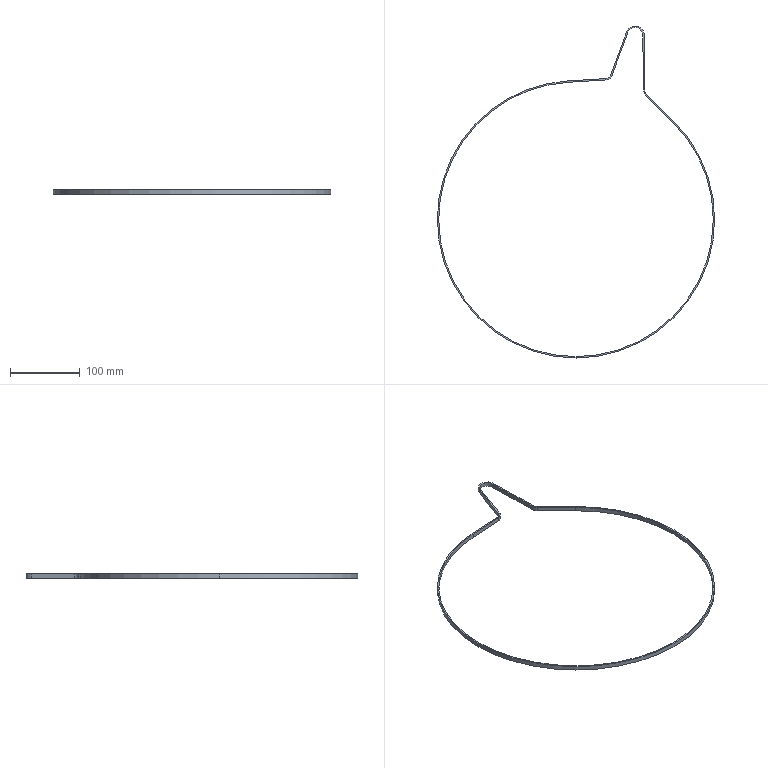Part | NX | features BREP 1 | 1 solid | 22 faces | box 398.69 x 477.38 x 6 mm | volume 16623 mm3 | cylinder 12 | plane 10 | commonest cylinder face diameters 394.69 x3 398.69 x3 17 x2 21 x2 22.07 x1 26.07 x1
STEP:
#1=CARTESIAN_POINT('',(42.641,200.38,-3.));
#2=VERTEX_POINT('',#1);
#3=CARTESIAN_POINT('',(-12.257,196.964,-3.));
#4=VERTEX_POINT('',#3);
#5=CARTESIAN_POINT('',(-12.257,196.964,-3.));
#6=DIRECTION('',(-0.9981,-0.06211,0.));
#7=VECTOR('',#6,1000.);
#8=LINE('',#5,#7);
#9=EDGE_CURVE('',#2,#4,#8,.T.);
#10=ORIENTED_EDGE('',*,*,#9,.F.);
#11=CARTESIAN_POINT('',(42.641,200.38,3.));
#12=VERTEX_POINT('',#11);
#13=CARTESIAN_POINT('',(42.641,200.38,3.));
#14=DIRECTION('',(0.,0.,-1.));
#15=VECTOR('',#14,1000.);
#16=LINE('',#13,#15);
#17=EDGE_CURVE('',#12,#2,#16,.T.);
#18=ORIENTED_EDGE('',*,*,#17,.F.);
#19=CARTESIAN_POINT('',(-12.257,196.964,3.));
#20=VERTEX_POINT('',#19);
#21=CARTESIAN_POINT('',(-12.257,196.964,3.));
#22=DIRECTION('',(-0.9981,-0.06211,0.));
#23=VECTOR('',#22,1000.);
#24=LINE('',#21,#23);
#25=EDGE_CURVE('',#12,#20,#24,.T.);
#26=ORIENTED_EDGE('',*,*,#25,.T.);
#27=CARTESIAN_POINT('',(-12.257,196.964,3.));
#28=DIRECTION('',(0.,0.,-1.));
#29=VECTOR('',#28,1000.);
#30=LINE('',#27,#29);
#31=EDGE_CURVE('',#20,#4,#30,.T.);
#32=ORIENTED_EDGE('',*,*,#31,.T.);
#33=EDGE_LOOP('',(#10,#18,#26,#32));
#34=FACE_BOUND('',#33,.T.);
#35=CARTESIAN_POINT('',(-12.257,196.964,3.));
#36=DIRECTION('',(0.06211,-0.9981,0.));
#37=DIRECTION('',(0.9981,0.06211,0.));
#38=AXIS2_PLACEMENT_3D('',#35,#36,#37);
#39=PLANE('',#38);
#40=ADVANCED_FACE('',(#34),#39,.T.);
#41=CARTESIAN_POINT('',(51.836,207.214,-3.));
#42=VERTEX_POINT('',#41);
#43=CARTESIAN_POINT('',(41.989,210.86,-3.));
#44=DIRECTION('',(0.,0.,-1.));
#45=DIRECTION('',(-1.,0.,0.));
#46=AXIS2_PLACEMENT_3D('',#43,#44,#45);
#47=CIRCLE('',#46,10.5);
#48=EDGE_CURVE('',#42,#2,#47,.T.);
#49=ORIENTED_EDGE('',*,*,#48,.F.);
#50=CARTESIAN_POINT('',(51.836,207.214,3.));
#51=VERTEX_POINT('',#50);
#52=CARTESIAN_POINT('',(51.836,207.214,3.));
#53=DIRECTION('',(0.,0.,-1.));
#54=VECTOR('',#53,1000.);
#55=LINE('',#52,#54);
#56=EDGE_CURVE('',#51,#42,#55,.T.);
#57=ORIENTED_EDGE('',*,*,#56,.F.);
#58=CARTESIAN_POINT('',(41.989,210.86,3.));
#59=DIRECTION('',(0.,0.,-1.));
#60=DIRECTION('',(-1.,0.,0.));
#61=AXIS2_PLACEMENT_3D('',#58,#59,#60);
#62=CIRCLE('',#61,10.5);
#63=EDGE_CURVE('',#51,#12,#62,.T.);
#64=ORIENTED_EDGE('',*,*,#63,.T.);
#65=ORIENTED_EDGE('',*,*,#17,.T.);
#66=EDGE_LOOP('',(#49,#57,#64,#65));
#67=FACE_BOUND('',#66,.T.);
#68=CARTESIAN_POINT('',(41.989,210.86,3.));
#69=DIRECTION('',(0.,0.,-1.));
#70=DIRECTION('',(-1.,0.,0.));
#71=AXIS2_PLACEMENT_3D('',#68,#69,#70);
#72=CYLINDRICAL_SURFACE('',#71,10.5);
#73=ADVANCED_FACE('',(#67),#72,.T.);
#74=CARTESIAN_POINT('',(74.652,268.832,-3.));
#75=VERTEX_POINT('',#74);
#76=CARTESIAN_POINT('',(-21.89,8.105,-3.));
#77=DIRECTION('',(-0.3472,-0.9378,0.));
#78=VECTOR('',#77,1000.);
#79=LINE('',#76,#78);
#80=EDGE_CURVE('',#75,#42,#79,.T.);
#81=ORIENTED_EDGE('',*,*,#80,.F.);
#82=CARTESIAN_POINT('',(74.652,268.832,3.));
#83=VERTEX_POINT('',#82);
#84=CARTESIAN_POINT('',(74.652,268.832,3.));
#85=DIRECTION('',(0.,0.,-1.));
#86=VECTOR('',#85,1000.);
#87=LINE('',#84,#86);
#88=EDGE_CURVE('',#83,#75,#87,.T.);
#89=ORIENTED_EDGE('',*,*,#88,.F.);
#90=CARTESIAN_POINT('',(-21.89,8.105,3.));
#91=DIRECTION('',(-0.3472,-0.9378,0.));
#92=VECTOR('',#91,1000.);
#93=LINE('',#90,#92);
#94=EDGE_CURVE('',#83,#51,#93,.T.);
#95=ORIENTED_EDGE('',*,*,#94,.T.);
#96=ORIENTED_EDGE('',*,*,#56,.T.);
#97=EDGE_LOOP('',(#81,#89,#95,#96));
#98=FACE_BOUND('',#97,.T.);
#99=CARTESIAN_POINT('',(-21.89,8.105,3.));
#100=DIRECTION('',(0.9378,-0.3472,0.));
#101=DIRECTION('',(0.3472,0.9378,0.));
#102=AXIS2_PLACEMENT_3D('',#99,#100,#101);
#103=PLANE('',#102);
#104=ADVANCED_FACE('',(#98),#103,.T.);
#105=CARTESIAN_POINT('',(96.034,265.135,-3.));
#106=VERTEX_POINT('',#105);
#107=CARTESIAN_POINT('',(85.,265.,-3.));
#108=DIRECTION('',(0.,0.,1.));
#109=DIRECTION('',(-1.,0.,0.));
#110=AXIS2_PLACEMENT_3D('',#107,#108,#109);
#111=CIRCLE('',#110,11.035);
#112=EDGE_CURVE('',#106,#75,#111,.T.);
#113=ORIENTED_EDGE('',*,*,#112,.F.);
#114=CARTESIAN_POINT('',(96.034,265.135,3.));
#115=VERTEX_POINT('',#114);
#116=CARTESIAN_POINT('',(96.034,265.135,3.));
#117=DIRECTION('',(0.,0.,-1.));
#118=VECTOR('',#117,1000.);
#119=LINE('',#116,#118);
#120=EDGE_CURVE('',#115,#106,#119,.T.);
#121=ORIENTED_EDGE('',*,*,#120,.F.);
#122=CARTESIAN_POINT('',(85.,265.,3.));
#123=DIRECTION('',(0.,0.,1.));
#124=DIRECTION('',(-1.,0.,0.));
#125=AXIS2_PLACEMENT_3D('',#122,#123,#124);
#126=CIRCLE('',#125,11.035);
#127=EDGE_CURVE('',#115,#83,#126,.T.);
#128=ORIENTED_EDGE('',*,*,#127,.T.);
#129=ORIENTED_EDGE('',*,*,#88,.T.);
#130=EDGE_LOOP('',(#113,#121,#128,#129));
#131=FACE_BOUND('',#130,.T.);
#132=CARTESIAN_POINT('',(85.,265.,3.));
#133=DIRECTION('',(0.,0.,-1.));
#134=DIRECTION('',(-1.,0.,0.));
#135=AXIS2_PLACEMENT_3D('',#132,#133,#134);
#136=CYLINDRICAL_SURFACE('',#135,11.035);
#137=ADVANCED_FACE('',(#131),#136,.F.);
#138=CARTESIAN_POINT('',(97.001,186.067,-3.));
#139=VERTEX_POINT('',#138);
#140=CARTESIAN_POINT('',(99.261,1.213,-3.));
#141=DIRECTION('',(-0.01222,0.9999,0.));
#142=VECTOR('',#141,1000.);
#143=LINE('',#140,#142);
#144=EDGE_CURVE('',#139,#106,#143,.T.);
#145=ORIENTED_EDGE('',*,*,#144,.F.);
#146=CARTESIAN_POINT('',(97.001,186.067,3.));
#147=VERTEX_POINT('',#146);
#148=CARTESIAN_POINT('',(97.001,186.067,3.));
#149=DIRECTION('',(0.,0.,-1.));
#150=VECTOR('',#149,1000.);
#151=LINE('',#148,#150);
#152=EDGE_CURVE('',#147,#139,#151,.T.);
#153=ORIENTED_EDGE('',*,*,#152,.F.);
#154=CARTESIAN_POINT('',(99.261,1.213,3.));
#155=DIRECTION('',(-0.01222,0.9999,0.));
#156=VECTOR('',#155,1000.);
#157=LINE('',#154,#156);
#158=EDGE_CURVE('',#147,#115,#157,.T.);
#159=ORIENTED_EDGE('',*,*,#158,.T.);
#160=ORIENTED_EDGE('',*,*,#120,.T.);
#161=EDGE_LOOP('',(#145,#153,#159,#160));
#162=FACE_BOUND('',#161,.T.);
#163=CARTESIAN_POINT('',(99.261,1.213,3.));
#164=DIRECTION('',(-0.9999,-0.01222,0.));
#165=DIRECTION('',(0.01222,-0.9999,0.));
#166=AXIS2_PLACEMENT_3D('',#163,#164,#165);
#167=PLANE('',#166);
#168=ADVANCED_FACE('',(#162),#167,.T.);
#169=CARTESIAN_POINT('',(100.098,178.748,-3.));
#170=VERTEX_POINT('',#169);
#171=CARTESIAN_POINT('',(107.5,186.195,-3.));
#172=DIRECTION('',(0.,0.,-1.));
#173=DIRECTION('',(-1.,0.,0.));
#174=AXIS2_PLACEMENT_3D('',#171,#172,#173);
#175=CIRCLE('',#174,10.5);
#176=EDGE_CURVE('',#170,#139,#175,.T.);
#177=ORIENTED_EDGE('',*,*,#176,.F.);
#178=CARTESIAN_POINT('',(100.098,178.748,3.));
#179=VERTEX_POINT('',#178);
#180=CARTESIAN_POINT('',(100.098,178.748,3.));
#181=DIRECTION('',(0.,0.,-1.));
#182=VECTOR('',#181,1000.);
#183=LINE('',#180,#182);
#184=EDGE_CURVE('',#179,#170,#183,.T.);
#185=ORIENTED_EDGE('',*,*,#184,.F.);
#186=CARTESIAN_POINT('',(107.5,186.195,3.));
#187=DIRECTION('',(0.,0.,-1.));
#188=DIRECTION('',(-1.,0.,0.));
#189=AXIS2_PLACEMENT_3D('',#186,#187,#188);
#190=CIRCLE('',#189,10.5);
#191=EDGE_CURVE('',#179,#147,#190,.T.);
#192=ORIENTED_EDGE('',*,*,#191,.T.);
#193=ORIENTED_EDGE('',*,*,#152,.T.);
#194=EDGE_LOOP('',(#177,#185,#192,#193));
#195=FACE_BOUND('',#194,.T.);
#196=CARTESIAN_POINT('',(107.5,186.195,3.));
#197=DIRECTION('',(0.,0.,-1.));
#198=DIRECTION('',(-1.,0.,0.));
#199=AXIS2_PLACEMENT_3D('',#196,#197,#198);
#200=CYLINDRICAL_SURFACE('',#199,10.5);
#201=ADVANCED_FACE('',(#195),#200,.T.);
#202=CARTESIAN_POINT('',(139.112,139.974,-3.));
#203=VERTEX_POINT('',#202);
#204=CARTESIAN_POINT('',(139.112,139.974,-3.));
#205=DIRECTION('',(-0.7093,0.7049,0.));
#206=VECTOR('',#205,1000.);
#207=LINE('',#204,#206);
#208=EDGE_CURVE('',#203,#170,#207,.T.);
#209=ORIENTED_EDGE('',*,*,#208,.F.);
#210=CARTESIAN_POINT('',(139.112,139.974,3.));
#211=VERTEX_POINT('',#210);
#212=CARTESIAN_POINT('',(139.112,139.974,3.));
#213=DIRECTION('',(0.,0.,-1.));
#214=VECTOR('',#213,1000.);
#215=LINE('',#212,#214);
#216=EDGE_CURVE('',#211,#203,#215,.T.);
#217=ORIENTED_EDGE('',*,*,#216,.F.);
#218=CARTESIAN_POINT('',(139.112,139.974,3.));
#219=DIRECTION('',(-0.7093,0.7049,0.));
#220=VECTOR('',#219,1000.);
#221=LINE('',#218,#220);
#222=EDGE_CURVE('',#211,#179,#221,.T.);
#223=ORIENTED_EDGE('',*,*,#222,.T.);
#224=ORIENTED_EDGE('',*,*,#184,.T.);
#225=EDGE_LOOP('',(#209,#217,#223,#224));
#226=FACE_BOUND('',#225,.T.);
#227=CARTESIAN_POINT('',(139.112,139.974,3.));
#228=DIRECTION('',(-0.7049,-0.7093,0.));
#229=DIRECTION('',(0.7093,-0.7049,0.));
#230=AXIS2_PLACEMENT_3D('',#227,#228,#229);
#231=PLANE('',#230);
#232=ADVANCED_FACE('',(#226),#231,.T.);
#233=CARTESIAN_POINT('',(197.345,0.,3.));
#234=VERTEX_POINT('',#233);
#235=CARTESIAN_POINT('',(197.345,0.,-3.));
#236=VERTEX_POINT('',#235);
#237=CARTESIAN_POINT('',(197.345,0.,3.));
#238=DIRECTION('',(0.,0.,-1.));
#239=VECTOR('',#238,1000.);
#240=LINE('',#237,#239);
#241=EDGE_CURVE('',#234,#236,#240,.T.);
#242=ORIENTED_EDGE('',*,*,#241,.F.);
#243=CARTESIAN_POINT('',(0.,0.,3.));
#244=DIRECTION('',(0.,0.,1.));
#245=DIRECTION('',(-1.,0.,0.));
#246=AXIS2_PLACEMENT_3D('',#243,#244,#245);
#247=CIRCLE('',#246,197.345);
#248=EDGE_CURVE('',#234,#211,#247,.T.);
#249=ORIENTED_EDGE('',*,*,#248,.T.);
#250=ORIENTED_EDGE('',*,*,#216,.T.);
#251=CARTESIAN_POINT('',(0.,0.,-3.));
#252=DIRECTION('',(0.,0.,1.));
#253=DIRECTION('',(-1.,0.,0.));
#254=AXIS2_PLACEMENT_3D('',#251,#252,#253);
#255=CIRCLE('',#254,197.345);
#256=EDGE_CURVE('',#236,#203,#255,.T.);
#257=ORIENTED_EDGE('',*,*,#256,.F.);
#258=EDGE_LOOP('',(#242,#249,#250,#257));
#259=FACE_BOUND('',#258,.T.);
#260=CARTESIAN_POINT('',(0.,0.,3.));
#261=DIRECTION('',(0.,0.,-1.));
#262=DIRECTION('',(-1.,0.,0.));
#263=AXIS2_PLACEMENT_3D('',#260,#261,#262);
#264=CYLINDRICAL_SURFACE('',#263,197.345);
#265=ADVANCED_FACE('',(#259),#264,.F.);
#266=CARTESIAN_POINT('',(42.517,202.376,-3.));
#267=VERTEX_POINT('',#266);
#268=CARTESIAN_POINT('',(-12.381,198.96,-3.));
#269=VERTEX_POINT('',#268);
#270=CARTESIAN_POINT('',(-12.381,198.96,-3.));
#271=DIRECTION('',(-0.9981,-0.06211,0.));
#272=VECTOR('',#271,1000.);
#273=LINE('',#270,#272);
#274=EDGE_CURVE('',#267,#269,#273,.T.);
#275=ORIENTED_EDGE('',*,*,#274,.T.);
#276=CARTESIAN_POINT('',(-12.381,198.96,3.));
#277=VERTEX_POINT('',#276);
#278=CARTESIAN_POINT('',(-12.381,198.96,3.));
#279=DIRECTION('',(0.,0.,-1.));
#280=VECTOR('',#279,1000.);
#281=LINE('',#278,#280);
#282=EDGE_CURVE('',#277,#269,#281,.T.);
#283=ORIENTED_EDGE('',*,*,#282,.F.);
#284=CARTESIAN_POINT('',(42.517,202.376,3.));
#285=VERTEX_POINT('',#284);
#286=CARTESIAN_POINT('',(-12.381,198.96,3.));
#287=DIRECTION('',(-0.9981,-0.06211,0.));
#288=VECTOR('',#287,1000.);
#289=LINE('',#286,#288);
#290=EDGE_CURVE('',#285,#277,#289,.T.);
#291=ORIENTED_EDGE('',*,*,#290,.F.);
#292=CARTESIAN_POINT('',(42.517,202.376,3.));
#293=DIRECTION('',(0.,0.,-1.));
#294=VECTOR('',#293,1000.);
#295=LINE('',#292,#294);
#296=EDGE_CURVE('',#285,#267,#295,.T.);
#297=ORIENTED_EDGE('',*,*,#296,.T.);
#298=EDGE_LOOP('',(#275,#283,#291,#297));
#299=FACE_BOUND('',#298,.T.);
#300=CARTESIAN_POINT('',(-12.381,198.96,3.));
#301=DIRECTION('',(0.06211,-0.9981,0.));
#302=DIRECTION('',(0.9981,0.06211,0.));
#303=AXIS2_PLACEMENT_3D('',#300,#301,#302);
#304=PLANE('',#303);
#305=ADVANCED_FACE('',(#299),#304,.F.);
#306=CARTESIAN_POINT('',(49.96,207.908,-3.));
#307=VERTEX_POINT('',#306);
#308=CARTESIAN_POINT('',(41.989,210.86,-3.));
#309=DIRECTION('',(0.,0.,-1.));
#310=DIRECTION('',(-1.,0.,0.));
#311=AXIS2_PLACEMENT_3D('',#308,#309,#310);
#312=CIRCLE('',#311,8.5);
#313=EDGE_CURVE('',#307,#267,#312,.T.);
#314=ORIENTED_EDGE('',*,*,#313,.T.);
#315=ORIENTED_EDGE('',*,*,#296,.F.);
#316=CARTESIAN_POINT('',(49.96,207.908,3.));
#317=VERTEX_POINT('',#316);
#318=CARTESIAN_POINT('',(41.989,210.86,3.));
#319=DIRECTION('',(0.,0.,-1.));
#320=DIRECTION('',(-1.,0.,0.));
#321=AXIS2_PLACEMENT_3D('',#318,#319,#320);
#322=CIRCLE('',#321,8.5);
#323=EDGE_CURVE('',#317,#285,#322,.T.);
#324=ORIENTED_EDGE('',*,*,#323,.F.);
#325=CARTESIAN_POINT('',(49.96,207.908,3.));
#326=DIRECTION('',(0.,0.,-1.));
#327=VECTOR('',#326,1000.);
#328=LINE('',#325,#327);
#329=EDGE_CURVE('',#317,#307,#328,.T.);
#330=ORIENTED_EDGE('',*,*,#329,.T.);
#331=EDGE_LOOP('',(#314,#315,#324,#330));
#332=FACE_BOUND('',#331,.T.);
#333=CARTESIAN_POINT('',(41.989,210.86,3.));
#334=DIRECTION('',(0.,0.,-1.));
#335=DIRECTION('',(-1.,0.,0.));
#336=AXIS2_PLACEMENT_3D('',#333,#334,#335);
#337=CYLINDRICAL_SURFACE('',#336,8.5);
#338=ADVANCED_FACE('',(#332),#337,.F.);
#339=CARTESIAN_POINT('',(72.776,269.526,-3.));
#340=VERTEX_POINT('',#339);
#341=CARTESIAN_POINT('',(-23.765,8.8,-3.));
#342=DIRECTION('',(-0.3472,-0.9378,0.));
#343=VECTOR('',#342,1000.);
#344=LINE('',#341,#343);
#345=EDGE_CURVE('',#340,#307,#344,.T.);
#346=ORIENTED_EDGE('',*,*,#345,.T.);
#347=ORIENTED_EDGE('',*,*,#329,.F.);
#348=CARTESIAN_POINT('',(72.776,269.526,3.));
#349=VERTEX_POINT('',#348);
#350=CARTESIAN_POINT('',(-23.765,8.8,3.));
#351=DIRECTION('',(-0.3472,-0.9378,0.));
#352=VECTOR('',#351,1000.);
#353=LINE('',#350,#352);
#354=EDGE_CURVE('',#349,#317,#353,.T.);
#355=ORIENTED_EDGE('',*,*,#354,.F.);
#356=CARTESIAN_POINT('',(72.776,269.526,3.));
#357=DIRECTION('',(0.,0.,-1.));
#358=VECTOR('',#357,1000.);
#359=LINE('',#356,#358);
#360=EDGE_CURVE('',#349,#340,#359,.T.);
#361=ORIENTED_EDGE('',*,*,#360,.T.);
#362=EDGE_LOOP('',(#346,#347,#355,#361));
#363=FACE_BOUND('',#362,.T.);
#364=CARTESIAN_POINT('',(-23.765,8.8,3.));
#365=DIRECTION('',(0.9378,-0.3472,0.));
#366=DIRECTION('',(0.3472,0.9378,0.));
#367=AXIS2_PLACEMENT_3D('',#364,#365,#366);
#368=PLANE('',#367);
#369=ADVANCED_FACE('',(#363),#368,.F.);
#370=CARTESIAN_POINT('',(98.034,265.159,-3.));
#371=VERTEX_POINT('',#370);
#372=CARTESIAN_POINT('',(85.,265.,-3.));
#373=DIRECTION('',(0.,0.,1.));
#374=DIRECTION('',(-1.,0.,0.));
#375=AXIS2_PLACEMENT_3D('',#372,#373,#374);
#376=CIRCLE('',#375,13.035);
#377=EDGE_CURVE('',#371,#340,#376,.T.);
#378=ORIENTED_EDGE('',*,*,#377,.T.);
#379=ORIENTED_EDGE('',*,*,#360,.F.);
#380=CARTESIAN_POINT('',(98.034,265.159,3.));
#381=VERTEX_POINT('',#380);
#382=CARTESIAN_POINT('',(85.,265.,3.));
#383=DIRECTION('',(0.,0.,1.));
#384=DIRECTION('',(-1.,0.,0.));
#385=AXIS2_PLACEMENT_3D('',#382,#383,#384);
#386=CIRCLE('',#385,13.035);
#387=EDGE_CURVE('',#381,#349,#386,.T.);
#388=ORIENTED_EDGE('',*,*,#387,.F.);
#389=CARTESIAN_POINT('',(98.034,265.159,3.));
#390=DIRECTION('',(0.,0.,-1.));
#391=VECTOR('',#390,1000.);
#392=LINE('',#389,#391);
#393=EDGE_CURVE('',#381,#371,#392,.T.);
#394=ORIENTED_EDGE('',*,*,#393,.T.);
#395=EDGE_LOOP('',(#378,#379,#388,#394));
#396=FACE_BOUND('',#395,.T.);
#397=CARTESIAN_POINT('',(85.,265.,3.));
#398=DIRECTION('',(0.,0.,-1.));
#399=DIRECTION('',(-1.,0.,0.));
#400=AXIS2_PLACEMENT_3D('',#397,#398,#399);
#401=CYLINDRICAL_SURFACE('',#400,13.035);
#402=ADVANCED_FACE('',(#396),#401,.T.);
#403=CARTESIAN_POINT('',(99.001,186.092,-3.));
#404=VERTEX_POINT('',#403);
#405=CARTESIAN_POINT('',(101.26,1.238,-3.));
#406=DIRECTION('',(-0.01222,0.9999,0.));
#407=VECTOR('',#406,1000.);
#408=LINE('',#405,#407);
#409=EDGE_CURVE('',#404,#371,#408,.T.);
#410=ORIENTED_EDGE('',*,*,#409,.T.);
#411=ORIENTED_EDGE('',*,*,#393,.F.);
#412=CARTESIAN_POINT('',(99.001,186.092,3.));
#413=VERTEX_POINT('',#412);
#414=CARTESIAN_POINT('',(101.26,1.238,3.));
#415=DIRECTION('',(-0.01222,0.9999,0.));
#416=VECTOR('',#415,1000.);
#417=LINE('',#414,#416);
#418=EDGE_CURVE('',#413,#381,#417,.T.);
#419=ORIENTED_EDGE('',*,*,#418,.F.);
#420=CARTESIAN_POINT('',(99.001,186.092,3.));
#421=DIRECTION('',(0.,0.,-1.));
#422=VECTOR('',#421,1000.);
#423=LINE('',#420,#422);
#424=EDGE_CURVE('',#413,#404,#423,.T.);
#425=ORIENTED_EDGE('',*,*,#424,.T.);
#426=EDGE_LOOP('',(#410,#411,#419,#425));
#427=FACE_BOUND('',#426,.T.);
#428=CARTESIAN_POINT('',(101.26,1.238,3.));
#429=DIRECTION('',(-0.9999,-0.01222,0.));
#430=DIRECTION('',(0.01222,-0.9999,0.));
#431=AXIS2_PLACEMENT_3D('',#428,#429,#430);
#432=PLANE('',#431);
#433=ADVANCED_FACE('',(#427),#432,.F.);
#434=CARTESIAN_POINT('',(101.508,180.167,-3.));
#435=VERTEX_POINT('',#434);
#436=CARTESIAN_POINT('',(107.5,186.195,-3.));
#437=DIRECTION('',(0.,0.,-1.));
#438=DIRECTION('',(-1.,0.,0.));
#439=AXIS2_PLACEMENT_3D('',#436,#437,#438);
#440=CIRCLE('',#439,8.5);
#441=EDGE_CURVE('',#435,#404,#440,.T.);
#442=ORIENTED_EDGE('',*,*,#441,.T.);
#443=ORIENTED_EDGE('',*,*,#424,.F.);
#444=CARTESIAN_POINT('',(101.508,180.167,3.));
#445=VERTEX_POINT('',#444);
#446=CARTESIAN_POINT('',(107.5,186.195,3.));
#447=DIRECTION('',(0.,0.,-1.));
#448=DIRECTION('',(-1.,0.,0.));
#449=AXIS2_PLACEMENT_3D('',#446,#447,#448);
#450=CIRCLE('',#449,8.5);
#451=EDGE_CURVE('',#445,#413,#450,.T.);
#452=ORIENTED_EDGE('',*,*,#451,.F.);
#453=CARTESIAN_POINT('',(101.508,180.167,3.));
#454=DIRECTION('',(0.,0.,-1.));
#455=VECTOR('',#454,1000.);
#456=LINE('',#453,#455);
#457=EDGE_CURVE('',#445,#435,#456,.T.);
#458=ORIENTED_EDGE('',*,*,#457,.T.);
#459=EDGE_LOOP('',(#442,#443,#452,#458));
#460=FACE_BOUND('',#459,.T.);
#461=CARTESIAN_POINT('',(107.5,186.195,3.));
#462=DIRECTION('',(0.,0.,-1.));
#463=DIRECTION('',(-1.,0.,0.));
#464=AXIS2_PLACEMENT_3D('',#461,#462,#463);
#465=CYLINDRICAL_SURFACE('',#464,8.5);
#466=ADVANCED_FACE('',(#460),#465,.F.);
#467=CARTESIAN_POINT('',(140.522,141.393,-3.));
#468=VERTEX_POINT('',#467);
#469=CARTESIAN_POINT('',(140.522,141.393,-3.));
#470=DIRECTION('',(-0.7093,0.7049,0.));
#471=VECTOR('',#470,1000.);
#472=LINE('',#469,#471);
#473=EDGE_CURVE('',#468,#435,#472,.T.);
#474=ORIENTED_EDGE('',*,*,#473,.T.);
#475=ORIENTED_EDGE('',*,*,#457,.F.);
#476=CARTESIAN_POINT('',(140.522,141.393,3.));
#477=VERTEX_POINT('',#476);
#478=CARTESIAN_POINT('',(140.522,141.393,3.));
#479=DIRECTION('',(-0.7093,0.7049,0.));
#480=VECTOR('',#479,1000.);
#481=LINE('',#478,#480);
#482=EDGE_CURVE('',#477,#445,#481,.T.);
#483=ORIENTED_EDGE('',*,*,#482,.F.);
#484=CARTESIAN_POINT('',(140.522,141.393,3.));
#485=DIRECTION('',(0.,0.,-1.));
#486=VECTOR('',#485,1000.);
#487=LINE('',#484,#486);
#488=EDGE_CURVE('',#477,#468,#487,.T.);
#489=ORIENTED_EDGE('',*,*,#488,.T.);
#490=EDGE_LOOP('',(#474,#475,#483,#489));
#491=FACE_BOUND('',#490,.T.);
#492=CARTESIAN_POINT('',(140.522,141.393,3.));
#493=DIRECTION('',(-0.7049,-0.7093,0.));
#494=DIRECTION('',(0.7093,-0.7049,0.));
#495=AXIS2_PLACEMENT_3D('',#492,#493,#494);
#496=PLANE('',#495);
#497=ADVANCED_FACE('',(#491),#496,.F.);
#498=CARTESIAN_POINT('',(-199.345,0.,3.));
#499=VERTEX_POINT('',#498);
#500=CARTESIAN_POINT('',(-199.345,0.,-3.));
#501=VERTEX_POINT('',#500);
#502=CARTESIAN_POINT('',(-199.345,0.,3.));
#503=DIRECTION('',(0.,0.,-1.));
#504=VECTOR('',#503,1000.);
#505=LINE('',#502,#504);
#506=EDGE_CURVE('',#499,#501,#505,.T.);
#507=ORIENTED_EDGE('',*,*,#506,.F.);
#508=CARTESIAN_POINT('',(0.,0.,3.));
#509=DIRECTION('',(0.,0.,1.));
#510=DIRECTION('',(-1.,0.,0.));
#511=AXIS2_PLACEMENT_3D('',#508,#509,#510);
#512=CIRCLE('',#511,199.345);
#513=EDGE_CURVE('',#277,#499,#512,.T.);
#514=ORIENTED_EDGE('',*,*,#513,.F.);
#515=ORIENTED_EDGE('',*,*,#282,.T.);
#516=CARTESIAN_POINT('',(0.,0.,-3.));
#517=DIRECTION('',(0.,0.,1.));
#518=DIRECTION('',(-1.,0.,0.));
#519=AXIS2_PLACEMENT_3D('',#516,#517,#518);
#520=CIRCLE('',#519,199.345);
#521=EDGE_CURVE('',#269,#501,#520,.T.);
#522=ORIENTED_EDGE('',*,*,#521,.T.);
#523=EDGE_LOOP('',(#507,#514,#515,#522));
#524=FACE_BOUND('',#523,.T.);
#525=CARTESIAN_POINT('',(0.,0.,3.));
#526=DIRECTION('',(0.,0.,-1.));
#527=DIRECTION('',(-1.,0.,0.));
#528=AXIS2_PLACEMENT_3D('',#525,#526,#527);
#529=CYLINDRICAL_SURFACE('',#528,199.345);
#530=ADVANCED_FACE('',(#524),#529,.T.);
#531=ORIENTED_EDGE('',*,*,#9,.T.);
#532=CARTESIAN_POINT('',(-197.345,0.,-3.));
#533=VERTEX_POINT('',#532);
#534=CARTESIAN_POINT('',(0.,0.,-3.));
#535=DIRECTION('',(0.,0.,1.));
#536=DIRECTION('',(-1.,0.,0.));
#537=AXIS2_PLACEMENT_3D('',#534,#535,#536);
#538=CIRCLE('',#537,197.345);
#539=EDGE_CURVE('',#4,#533,#538,.T.);
#540=ORIENTED_EDGE('',*,*,#539,.T.);
#541=CARTESIAN_POINT('',(0.,0.,-3.));
#542=DIRECTION('',(0.,0.,1.));
#543=DIRECTION('',(-1.,0.,0.));
#544=AXIS2_PLACEMENT_3D('',#541,#542,#543);
#545=CIRCLE('',#544,197.345);
#546=EDGE_CURVE('',#533,#236,#545,.T.);
#547=ORIENTED_EDGE('',*,*,#546,.T.);
#548=ORIENTED_EDGE('',*,*,#256,.T.);
#549=ORIENTED_EDGE('',*,*,#208,.T.);
#550=ORIENTED_EDGE('',*,*,#176,.T.);
#551=ORIENTED_EDGE('',*,*,#144,.T.);
#552=ORIENTED_EDGE('',*,*,#112,.T.);
#553=ORIENTED_EDGE('',*,*,#80,.T.);
#554=ORIENTED_EDGE('',*,*,#48,.T.);
#555=EDGE_LOOP('',(#531,#540,#547,#548,#549,#550,#551,#552,#553,#554));
#556=FACE_BOUND('',#555,.T.);
#557=ORIENTED_EDGE('',*,*,#521,.F.);
#558=ORIENTED_EDGE('',*,*,#274,.F.);
#559=ORIENTED_EDGE('',*,*,#313,.F.);
#560=ORIENTED_EDGE('',*,*,#345,.F.);
#561=ORIENTED_EDGE('',*,*,#377,.F.);
#562=ORIENTED_EDGE('',*,*,#409,.F.);
#563=ORIENTED_EDGE('',*,*,#441,.F.);
#564=ORIENTED_EDGE('',*,*,#473,.F.);
#565=CARTESIAN_POINT('',(199.345,0.,-3.));
#566=VERTEX_POINT('',#565);
#567=CARTESIAN_POINT('',(0.,0.,-3.));
#568=DIRECTION('',(0.,0.,1.));
#569=DIRECTION('',(-1.,0.,0.));
#570=AXIS2_PLACEMENT_3D('',#567,#568,#569);
#571=CIRCLE('',#570,199.345);
#572=EDGE_CURVE('',#566,#468,#571,.T.);
#573=ORIENTED_EDGE('',*,*,#572,.F.);
#574=CARTESIAN_POINT('',(0.,0.,-3.));
#575=DIRECTION('',(0.,0.,1.));
#576=DIRECTION('',(-1.,0.,0.));
#577=AXIS2_PLACEMENT_3D('',#574,#575,#576);
#578=CIRCLE('',#577,199.345);
#579=EDGE_CURVE('',#501,#566,#578,.T.);
#580=ORIENTED_EDGE('',*,*,#579,.F.);
#581=EDGE_LOOP('',(#557,#558,#559,#560,#561,#562,#563,#564,#573,#580));
#582=FACE_BOUND('',#581,.T.);
#583=CARTESIAN_POINT('',(0.,0.,-3.));
#584=DIRECTION('',(0.,0.,-1.));
#585=DIRECTION('',(-1.,0.,0.));
#586=AXIS2_PLACEMENT_3D('',#583,#584,#585);
#587=PLANE('',#586);
#588=ADVANCED_FACE('',(#556,#582),#587,.T.);
#589=CARTESIAN_POINT('',(-197.345,0.,3.));
#590=VERTEX_POINT('',#589);
#591=CARTESIAN_POINT('',(0.,0.,3.));
#592=DIRECTION('',(0.,0.,1.));
#593=DIRECTION('',(-1.,0.,0.));
#594=AXIS2_PLACEMENT_3D('',#591,#592,#593);
#595=CIRCLE('',#594,197.345);
#596=EDGE_CURVE('',#20,#590,#595,.T.);
#597=ORIENTED_EDGE('',*,*,#596,.F.);
#598=ORIENTED_EDGE('',*,*,#25,.F.);
#599=ORIENTED_EDGE('',*,*,#63,.F.);
#600=ORIENTED_EDGE('',*,*,#94,.F.);
#601=ORIENTED_EDGE('',*,*,#127,.F.);
#602=ORIENTED_EDGE('',*,*,#158,.F.);
#603=ORIENTED_EDGE('',*,*,#191,.F.);
#604=ORIENTED_EDGE('',*,*,#222,.F.);
#605=ORIENTED_EDGE('',*,*,#248,.F.);
#606=CARTESIAN_POINT('',(0.,0.,3.));
#607=DIRECTION('',(0.,0.,1.));
#608=DIRECTION('',(-1.,0.,0.));
#609=AXIS2_PLACEMENT_3D('',#606,#607,#608);
#610=CIRCLE('',#609,197.345);
#611=EDGE_CURVE('',#590,#234,#610,.T.);
#612=ORIENTED_EDGE('',*,*,#611,.F.);
#613=EDGE_LOOP('',(#597,#598,#599,#600,#601,#602,#603,#604,#605,#612));
#614=FACE_BOUND('',#613,.T.);
#615=ORIENTED_EDGE('',*,*,#513,.T.);
#616=CARTESIAN_POINT('',(199.345,0.,3.));
#617=VERTEX_POINT('',#616);
#618=CARTESIAN_POINT('',(0.,0.,3.));
#619=DIRECTION('',(0.,0.,1.));
#620=DIRECTION('',(-1.,0.,0.));
#621=AXIS2_PLACEMENT_3D('',#618,#619,#620);
#622=CIRCLE('',#621,199.345);
#623=EDGE_CURVE('',#499,#617,#622,.T.);
#624=ORIENTED_EDGE('',*,*,#623,.T.);
#625=CARTESIAN_POINT('',(0.,0.,3.));
#626=DIRECTION('',(0.,0.,1.));
#627=DIRECTION('',(-1.,0.,0.));
#628=AXIS2_PLACEMENT_3D('',#625,#626,#627);
#629=CIRCLE('',#628,199.345);
#630=EDGE_CURVE('',#617,#477,#629,.T.);
#631=ORIENTED_EDGE('',*,*,#630,.T.);
#632=ORIENTED_EDGE('',*,*,#482,.T.);
#633=ORIENTED_EDGE('',*,*,#451,.T.);
#634=ORIENTED_EDGE('',*,*,#418,.T.);
#635=ORIENTED_EDGE('',*,*,#387,.T.);
#636=ORIENTED_EDGE('',*,*,#354,.T.);
#637=ORIENTED_EDGE('',*,*,#323,.T.);
#638=ORIENTED_EDGE('',*,*,#290,.T.);
#639=EDGE_LOOP('',(#615,#624,#631,#632,#633,#634,#635,#636,#637,#638));
#640=FACE_BOUND('',#639,.T.);
#641=CARTESIAN_POINT('',(0.,0.,3.));
#642=DIRECTION('',(0.,0.,-1.));
#643=DIRECTION('',(-1.,0.,0.));
#644=AXIS2_PLACEMENT_3D('',#641,#642,#643);
#645=PLANE('',#644);
#646=ADVANCED_FACE('',(#614,#640),#645,.F.);
#647=CARTESIAN_POINT('',(199.345,0.,3.));
#648=DIRECTION('',(0.,0.,-1.));
#649=VECTOR('',#648,1000.);
#650=LINE('',#647,#649);
#651=EDGE_CURVE('',#617,#566,#650,.T.);
#652=ORIENTED_EDGE('',*,*,#651,.F.);
#653=ORIENTED_EDGE('',*,*,#623,.F.);
#654=ORIENTED_EDGE('',*,*,#506,.T.);
#655=ORIENTED_EDGE('',*,*,#579,.T.);
#656=EDGE_LOOP('',(#652,#653,#654,#655));
#657=FACE_BOUND('',#656,.T.);
#658=CARTESIAN_POINT('',(0.,0.,3.));
#659=DIRECTION('',(0.,0.,-1.));
#660=DIRECTION('',(-1.,0.,0.));
#661=AXIS2_PLACEMENT_3D('',#658,#659,#660);
#662=CYLINDRICAL_SURFACE('',#661,199.345);
#663=ADVANCED_FACE('',(#657),#662,.T.);
#664=ORIENTED_EDGE('',*,*,#630,.F.);
#665=ORIENTED_EDGE('',*,*,#651,.T.);
#666=ORIENTED_EDGE('',*,*,#572,.T.);
#667=ORIENTED_EDGE('',*,*,#488,.F.);
#668=EDGE_LOOP('',(#664,#665,#666,#667));
#669=FACE_BOUND('',#668,.T.);
#670=CARTESIAN_POINT('',(0.,0.,3.));
#671=DIRECTION('',(0.,0.,-1.));
#672=DIRECTION('',(-1.,0.,0.));
#673=AXIS2_PLACEMENT_3D('',#670,#671,#672);
#674=CYLINDRICAL_SURFACE('',#673,199.345);
#675=ADVANCED_FACE('',(#669),#674,.T.);
#676=ORIENTED_EDGE('',*,*,#596,.T.);
#677=CARTESIAN_POINT('',(-197.345,0.,3.));
#678=DIRECTION('',(0.,0.,-1.));
#679=VECTOR('',#678,1000.);
#680=LINE('',#677,#679);
#681=EDGE_CURVE('',#590,#533,#680,.T.);
#682=ORIENTED_EDGE('',*,*,#681,.T.);
#683=ORIENTED_EDGE('',*,*,#539,.F.);
#684=ORIENTED_EDGE('',*,*,#31,.F.);
#685=EDGE_LOOP('',(#676,#682,#683,#684));
#686=FACE_BOUND('',#685,.T.);
#687=CARTESIAN_POINT('',(0.,0.,3.));
#688=DIRECTION('',(0.,0.,-1.));
#689=DIRECTION('',(-1.,0.,0.));
#690=AXIS2_PLACEMENT_3D('',#687,#688,#689);
#691=CYLINDRICAL_SURFACE('',#690,197.345);
#692=ADVANCED_FACE('',(#686),#691,.F.);
#693=ORIENTED_EDGE('',*,*,#611,.T.);
#694=ORIENTED_EDGE('',*,*,#241,.T.);
#695=ORIENTED_EDGE('',*,*,#546,.F.);
#696=ORIENTED_EDGE('',*,*,#681,.F.);
#697=EDGE_LOOP('',(#693,#694,#695,#696));
#698=FACE_BOUND('',#697,.T.);
#699=CARTESIAN_POINT('',(0.,0.,3.));
#700=DIRECTION('',(0.,0.,-1.));
#701=DIRECTION('',(-1.,0.,0.));
#702=AXIS2_PLACEMENT_3D('',#699,#700,#701);
#703=CYLINDRICAL_SURFACE('',#702,197.345);
#704=ADVANCED_FACE('',(#698),#703,.F.);
#705=CLOSED_SHELL('',(#40,#73,#104,#137,#168,#201,#232,#265,#305,#338,#369,#402,#433,#466,#497,#530,#588,#646,#663,#675,#692,#704));
#706=MANIFOLD_SOLID_BREP('',#705);
#707=(LENGTH_UNIT()NAMED_UNIT(*)SI_UNIT(.MILLI.,.METRE.));
#708=UNCERTAINTY_MEASURE_WITH_UNIT(LENGTH_MEASURE(0.00001),#707,'','');
#709=(NAMED_UNIT(*)PLANE_ANGLE_UNIT()SI_UNIT($,.RADIAN.));
#710=(NAMED_UNIT(*)SI_UNIT($,.STERADIAN.)SOLID_ANGLE_UNIT());
#711=(GEOMETRIC_REPRESENTATION_CONTEXT(3)GLOBAL_UNCERTAINTY_ASSIGNED_CONTEXT((#708))GLOBAL_UNIT_ASSIGNED_CONTEXT((#707,#709,#710))REPRESENTATION_CONTEXT('',''));
#712=ADVANCED_BREP_SHAPE_REPRESENTATION('',(#706),#711);